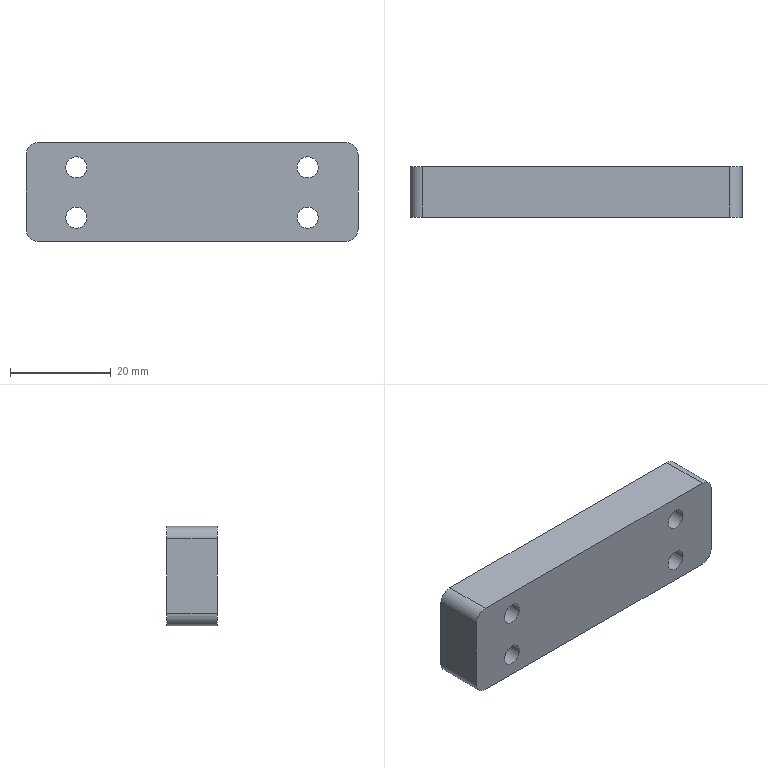Part | SolidWorks | features BaseBody 1 | 1 solid | 18 faces | box 66 x 10 x 19.75 mm | volume 12427 mm3 | cylinder 12 | plane 6 | commonest cylinder face diameters 4.2 x8 5 x4
STEP:
#1=CARTESIAN_POINT('',(-705.131,748.297,332.732));
#2=VERTEX_POINT('',#1);
#3=CARTESIAN_POINT('',(-702.631,748.297,335.232));
#4=VERTEX_POINT('',#3);
#5=CARTESIAN_POINT('',(-705.131,748.297,335.232));
#6=DIRECTION('',(0.,-1.,0.));
#7=DIRECTION('',(0.,0.,-1.));
#8=AXIS2_PLACEMENT_3D('',#5,#6,#7);
#9=CIRCLE('',#8,2.5);
#10=EDGE_CURVE('',#2,#4,#9,.T.);
#11=ORIENTED_EDGE('',*,*,#10,.F.);
#12=CARTESIAN_POINT('',(-766.131,748.297,332.732));
#13=VERTEX_POINT('',#12);
#14=CARTESIAN_POINT('',(-766.131,748.297,332.732));
#15=DIRECTION('',(1.,0.,0.));
#16=VECTOR('',#15,1000.);
#17=LINE('',#14,#16);
#18=EDGE_CURVE('',#13,#2,#17,.T.);
#19=ORIENTED_EDGE('',*,*,#18,.F.);
#20=CARTESIAN_POINT('',(-768.631,748.297,335.232));
#21=VERTEX_POINT('',#20);
#22=CARTESIAN_POINT('',(-766.131,748.297,335.232));
#23=DIRECTION('',(0.,-1.,0.));
#24=DIRECTION('',(-1.,0.,0.));
#25=AXIS2_PLACEMENT_3D('',#22,#23,#24);
#26=CIRCLE('',#25,2.5);
#27=EDGE_CURVE('',#21,#13,#26,.T.);
#28=ORIENTED_EDGE('',*,*,#27,.F.);
#29=CARTESIAN_POINT('',(-768.631,748.297,349.982));
#30=VERTEX_POINT('',#29);
#31=CARTESIAN_POINT('',(-768.631,748.297,349.982));
#32=DIRECTION('',(0.,0.,-1.));
#33=VECTOR('',#32,1000.);
#34=LINE('',#31,#33);
#35=EDGE_CURVE('',#30,#21,#34,.T.);
#36=ORIENTED_EDGE('',*,*,#35,.F.);
#37=CARTESIAN_POINT('',(-766.131,748.297,352.482));
#38=VERTEX_POINT('',#37);
#39=CARTESIAN_POINT('',(-766.131,748.297,349.982));
#40=DIRECTION('',(0.,-1.,0.));
#41=DIRECTION('',(0.,0.,1.));
#42=AXIS2_PLACEMENT_3D('',#39,#40,#41);
#43=CIRCLE('',#42,2.5);
#44=EDGE_CURVE('',#38,#30,#43,.T.);
#45=ORIENTED_EDGE('',*,*,#44,.F.);
#46=CARTESIAN_POINT('',(-705.131,748.297,352.482));
#47=VERTEX_POINT('',#46);
#48=CARTESIAN_POINT('',(-705.131,748.297,352.482));
#49=DIRECTION('',(-1.,0.,0.));
#50=VECTOR('',#49,1000.);
#51=LINE('',#48,#50);
#52=EDGE_CURVE('',#47,#38,#51,.T.);
#53=ORIENTED_EDGE('',*,*,#52,.F.);
#54=CARTESIAN_POINT('',(-702.631,748.297,349.982));
#55=VERTEX_POINT('',#54);
#56=CARTESIAN_POINT('',(-705.131,748.297,349.982));
#57=DIRECTION('',(0.,-1.,0.));
#58=DIRECTION('',(1.,0.,0.));
#59=AXIS2_PLACEMENT_3D('',#56,#57,#58);
#60=CIRCLE('',#59,2.5);
#61=EDGE_CURVE('',#55,#47,#60,.T.);
#62=ORIENTED_EDGE('',*,*,#61,.F.);
#63=CARTESIAN_POINT('',(-702.631,748.297,335.232));
#64=DIRECTION('',(0.,0.,1.));
#65=VECTOR('',#64,1000.);
#66=LINE('',#63,#65);
#67=EDGE_CURVE('',#4,#55,#66,.T.);
#68=ORIENTED_EDGE('',*,*,#67,.F.);
#69=EDGE_LOOP('',(#11,#19,#28,#36,#45,#53,#62,#68));
#70=FACE_OUTER_BOUND('',#69,.T.);
#71=CARTESIAN_POINT('',(-710.531,748.297,347.482));
#72=VERTEX_POINT('',#71);
#73=CARTESIAN_POINT('',(-714.731,748.297,347.482));
#74=VERTEX_POINT('',#73);
#75=CARTESIAN_POINT('',(-712.631,748.297,347.482));
#76=DIRECTION('',(0.,1.,0.));
#77=DIRECTION('',(1.,0.,0.));
#78=AXIS2_PLACEMENT_3D('',#75,#76,#77);
#79=CIRCLE('',#78,2.1);
#80=EDGE_CURVE('',#72,#74,#79,.T.);
#81=ORIENTED_EDGE('',*,*,#80,.F.);
#82=CARTESIAN_POINT('',(-712.631,748.297,347.482));
#83=DIRECTION('',(0.,1.,0.));
#84=DIRECTION('',(-1.,0.,0.));
#85=AXIS2_PLACEMENT_3D('',#82,#83,#84);
#86=CIRCLE('',#85,2.1);
#87=EDGE_CURVE('',#74,#72,#86,.T.);
#88=ORIENTED_EDGE('',*,*,#87,.F.);
#89=EDGE_LOOP('',(#81,#88));
#90=FACE_BOUND('',#89,.T.);
#91=CARTESIAN_POINT('',(-756.531,748.297,347.482));
#92=VERTEX_POINT('',#91);
#93=CARTESIAN_POINT('',(-760.731,748.297,347.482));
#94=VERTEX_POINT('',#93);
#95=CARTESIAN_POINT('',(-758.631,748.297,347.482));
#96=DIRECTION('',(0.,1.,0.));
#97=DIRECTION('',(1.,0.,0.));
#98=AXIS2_PLACEMENT_3D('',#95,#96,#97);
#99=CIRCLE('',#98,2.1);
#100=EDGE_CURVE('',#92,#94,#99,.T.);
#101=ORIENTED_EDGE('',*,*,#100,.F.);
#102=CARTESIAN_POINT('',(-758.631,748.297,347.482));
#103=DIRECTION('',(0.,1.,0.));
#104=DIRECTION('',(-1.,0.,0.));
#105=AXIS2_PLACEMENT_3D('',#102,#103,#104);
#106=CIRCLE('',#105,2.1);
#107=EDGE_CURVE('',#94,#92,#106,.T.);
#108=ORIENTED_EDGE('',*,*,#107,.F.);
#109=EDGE_LOOP('',(#101,#108));
#110=FACE_BOUND('',#109,.T.);
#111=CARTESIAN_POINT('',(-756.531,748.297,337.482));
#112=VERTEX_POINT('',#111);
#113=CARTESIAN_POINT('',(-760.731,748.297,337.482));
#114=VERTEX_POINT('',#113);
#115=CARTESIAN_POINT('',(-758.631,748.297,337.482));
#116=DIRECTION('',(0.,1.,0.));
#117=DIRECTION('',(1.,0.,0.));
#118=AXIS2_PLACEMENT_3D('',#115,#116,#117);
#119=CIRCLE('',#118,2.1);
#120=EDGE_CURVE('',#112,#114,#119,.T.);
#121=ORIENTED_EDGE('',*,*,#120,.F.);
#122=CARTESIAN_POINT('',(-758.631,748.297,337.482));
#123=DIRECTION('',(0.,1.,0.));
#124=DIRECTION('',(-1.,0.,0.));
#125=AXIS2_PLACEMENT_3D('',#122,#123,#124);
#126=CIRCLE('',#125,2.1);
#127=EDGE_CURVE('',#114,#112,#126,.T.);
#128=ORIENTED_EDGE('',*,*,#127,.F.);
#129=EDGE_LOOP('',(#121,#128));
#130=FACE_BOUND('',#129,.T.);
#131=CARTESIAN_POINT('',(-710.531,748.297,337.482));
#132=VERTEX_POINT('',#131);
#133=CARTESIAN_POINT('',(-714.731,748.297,337.482));
#134=VERTEX_POINT('',#133);
#135=CARTESIAN_POINT('',(-712.631,748.297,337.482));
#136=DIRECTION('',(0.,1.,0.));
#137=DIRECTION('',(1.,0.,0.));
#138=AXIS2_PLACEMENT_3D('',#135,#136,#137);
#139=CIRCLE('',#138,2.1);
#140=EDGE_CURVE('',#132,#134,#139,.T.);
#141=ORIENTED_EDGE('',*,*,#140,.F.);
#142=CARTESIAN_POINT('',(-712.631,748.297,337.482));
#143=DIRECTION('',(0.,1.,0.));
#144=DIRECTION('',(-1.,0.,0.));
#145=AXIS2_PLACEMENT_3D('',#142,#143,#144);
#146=CIRCLE('',#145,2.1);
#147=EDGE_CURVE('',#134,#132,#146,.T.);
#148=ORIENTED_EDGE('',*,*,#147,.F.);
#149=EDGE_LOOP('',(#141,#148));
#150=FACE_BOUND('',#149,.T.);
#151=CARTESIAN_POINT('',(-735.631,748.297,352.232));
#152=DIRECTION('',(0.,1.,0.));
#153=DIRECTION('',(-1.,0.,0.));
#154=AXIS2_PLACEMENT_3D('',#151,#152,#153);
#155=PLANE('',#154);
#156=ADVANCED_FACE('',(#70,#90,#110,#130,#150),#155,.T.);
#157=CARTESIAN_POINT('',(-702.631,738.297,335.232));
#158=VERTEX_POINT('',#157);
#159=CARTESIAN_POINT('',(-702.631,738.297,335.232));
#160=DIRECTION('',(0.,1.,0.));
#161=VECTOR('',#160,1000.);
#162=LINE('',#159,#161);
#163=EDGE_CURVE('',#158,#4,#162,.T.);
#164=ORIENTED_EDGE('',*,*,#163,.T.);
#165=ORIENTED_EDGE('',*,*,#67,.T.);
#166=CARTESIAN_POINT('',(-702.631,738.297,349.982));
#167=VERTEX_POINT('',#166);
#168=CARTESIAN_POINT('',(-702.631,748.297,349.982));
#169=DIRECTION('',(0.,-1.,0.));
#170=VECTOR('',#169,1000.);
#171=LINE('',#168,#170);
#172=EDGE_CURVE('',#55,#167,#171,.T.);
#173=ORIENTED_EDGE('',*,*,#172,.T.);
#174=CARTESIAN_POINT('',(-702.631,738.297,349.982));
#175=DIRECTION('',(0.,0.,-1.));
#176=VECTOR('',#175,1000.);
#177=LINE('',#174,#176);
#178=EDGE_CURVE('',#167,#158,#177,.T.);
#179=ORIENTED_EDGE('',*,*,#178,.T.);
#180=EDGE_LOOP('',(#164,#165,#173,#179));
#181=FACE_OUTER_BOUND('',#180,.T.);
#182=CARTESIAN_POINT('',(-702.631,748.297,364.732));
#183=DIRECTION('',(-1.,0.,0.));
#184=DIRECTION('',(0.,-1.,0.));
#185=AXIS2_PLACEMENT_3D('',#182,#183,#184);
#186=PLANE('',#185);
#187=ADVANCED_FACE('',(#181),#186,.F.);
#188=CARTESIAN_POINT('',(-768.631,738.297,349.982));
#189=VERTEX_POINT('',#188);
#190=CARTESIAN_POINT('',(-766.131,738.297,352.482));
#191=VERTEX_POINT('',#190);
#192=CARTESIAN_POINT('',(-766.131,738.297,349.982));
#193=DIRECTION('',(0.,1.,0.));
#194=DIRECTION('',(-1.,0.,0.));
#195=AXIS2_PLACEMENT_3D('',#192,#193,#194);
#196=CIRCLE('',#195,2.5);
#197=EDGE_CURVE('',#189,#191,#196,.T.);
#198=ORIENTED_EDGE('',*,*,#197,.F.);
#199=CARTESIAN_POINT('',(-768.631,738.297,335.232));
#200=VERTEX_POINT('',#199);
#201=CARTESIAN_POINT('',(-768.631,738.297,335.232));
#202=DIRECTION('',(0.,0.,1.));
#203=VECTOR('',#202,1000.);
#204=LINE('',#201,#203);
#205=EDGE_CURVE('',#200,#189,#204,.T.);
#206=ORIENTED_EDGE('',*,*,#205,.F.);
#207=CARTESIAN_POINT('',(-766.131,738.297,332.732));
#208=VERTEX_POINT('',#207);
#209=CARTESIAN_POINT('',(-766.131,738.297,335.232));
#210=DIRECTION('',(0.,1.,0.));
#211=DIRECTION('',(0.,0.,-1.));
#212=AXIS2_PLACEMENT_3D('',#209,#210,#211);
#213=CIRCLE('',#212,2.5);
#214=EDGE_CURVE('',#208,#200,#213,.T.);
#215=ORIENTED_EDGE('',*,*,#214,.F.);
#216=CARTESIAN_POINT('',(-705.131,738.297,332.732));
#217=VERTEX_POINT('',#216);
#218=CARTESIAN_POINT('',(-705.131,738.297,332.732));
#219=DIRECTION('',(-1.,0.,0.));
#220=VECTOR('',#219,1000.);
#221=LINE('',#218,#220);
#222=EDGE_CURVE('',#217,#208,#221,.T.);
#223=ORIENTED_EDGE('',*,*,#222,.F.);
#224=CARTESIAN_POINT('',(-705.131,738.297,335.232));
#225=DIRECTION('',(0.,1.,0.));
#226=DIRECTION('',(1.,0.,0.));
#227=AXIS2_PLACEMENT_3D('',#224,#225,#226);
#228=CIRCLE('',#227,2.5);
#229=EDGE_CURVE('',#158,#217,#228,.T.);
#230=ORIENTED_EDGE('',*,*,#229,.F.);
#231=ORIENTED_EDGE('',*,*,#178,.F.);
#232=CARTESIAN_POINT('',(-705.131,738.297,352.482));
#233=VERTEX_POINT('',#232);
#234=CARTESIAN_POINT('',(-705.131,738.297,349.982));
#235=DIRECTION('',(0.,1.,0.));
#236=DIRECTION('',(0.,0.,1.));
#237=AXIS2_PLACEMENT_3D('',#234,#235,#236);
#238=CIRCLE('',#237,2.5);
#239=EDGE_CURVE('',#233,#167,#238,.T.);
#240=ORIENTED_EDGE('',*,*,#239,.F.);
#241=CARTESIAN_POINT('',(-766.131,738.297,352.482));
#242=DIRECTION('',(1.,0.,0.));
#243=VECTOR('',#242,1000.);
#244=LINE('',#241,#243);
#245=EDGE_CURVE('',#191,#233,#244,.T.);
#246=ORIENTED_EDGE('',*,*,#245,.F.);
#247=EDGE_LOOP('',(#198,#206,#215,#223,#230,#231,#240,#246));
#248=FACE_OUTER_BOUND('',#247,.T.);
#249=CARTESIAN_POINT('',(-714.731,738.297,347.482));
#250=VERTEX_POINT('',#249);
#251=CARTESIAN_POINT('',(-710.531,738.297,347.482));
#252=VERTEX_POINT('',#251);
#253=CARTESIAN_POINT('',(-712.631,738.297,347.482));
#254=DIRECTION('',(0.,-1.,0.));
#255=DIRECTION('',(-1.,0.,0.));
#256=AXIS2_PLACEMENT_3D('',#253,#254,#255);
#257=CIRCLE('',#256,2.1);
#258=EDGE_CURVE('',#250,#252,#257,.T.);
#259=ORIENTED_EDGE('',*,*,#258,.F.);
#260=CARTESIAN_POINT('',(-712.631,738.297,347.482));
#261=DIRECTION('',(0.,-1.,0.));
#262=DIRECTION('',(1.,0.,0.));
#263=AXIS2_PLACEMENT_3D('',#260,#261,#262);
#264=CIRCLE('',#263,2.1);
#265=EDGE_CURVE('',#252,#250,#264,.T.);
#266=ORIENTED_EDGE('',*,*,#265,.F.);
#267=EDGE_LOOP('',(#259,#266));
#268=FACE_BOUND('',#267,.T.);
#269=CARTESIAN_POINT('',(-760.731,738.297,347.482));
#270=VERTEX_POINT('',#269);
#271=CARTESIAN_POINT('',(-756.531,738.297,347.482));
#272=VERTEX_POINT('',#271);
#273=CARTESIAN_POINT('',(-758.631,738.297,347.482));
#274=DIRECTION('',(0.,-1.,0.));
#275=DIRECTION('',(-1.,0.,0.));
#276=AXIS2_PLACEMENT_3D('',#273,#274,#275);
#277=CIRCLE('',#276,2.1);
#278=EDGE_CURVE('',#270,#272,#277,.T.);
#279=ORIENTED_EDGE('',*,*,#278,.F.);
#280=CARTESIAN_POINT('',(-758.631,738.297,347.482));
#281=DIRECTION('',(0.,-1.,0.));
#282=DIRECTION('',(1.,0.,0.));
#283=AXIS2_PLACEMENT_3D('',#280,#281,#282);
#284=CIRCLE('',#283,2.1);
#285=EDGE_CURVE('',#272,#270,#284,.T.);
#286=ORIENTED_EDGE('',*,*,#285,.F.);
#287=EDGE_LOOP('',(#279,#286));
#288=FACE_BOUND('',#287,.T.);
#289=CARTESIAN_POINT('',(-760.731,738.297,337.482));
#290=VERTEX_POINT('',#289);
#291=CARTESIAN_POINT('',(-756.531,738.297,337.482));
#292=VERTEX_POINT('',#291);
#293=CARTESIAN_POINT('',(-758.631,738.297,337.482));
#294=DIRECTION('',(0.,-1.,0.));
#295=DIRECTION('',(-1.,0.,0.));
#296=AXIS2_PLACEMENT_3D('',#293,#294,#295);
#297=CIRCLE('',#296,2.1);
#298=EDGE_CURVE('',#290,#292,#297,.T.);
#299=ORIENTED_EDGE('',*,*,#298,.F.);
#300=CARTESIAN_POINT('',(-758.631,738.297,337.482));
#301=DIRECTION('',(0.,-1.,0.));
#302=DIRECTION('',(1.,0.,0.));
#303=AXIS2_PLACEMENT_3D('',#300,#301,#302);
#304=CIRCLE('',#303,2.1);
#305=EDGE_CURVE('',#292,#290,#304,.T.);
#306=ORIENTED_EDGE('',*,*,#305,.F.);
#307=EDGE_LOOP('',(#299,#306));
#308=FACE_BOUND('',#307,.T.);
#309=CARTESIAN_POINT('',(-714.731,738.297,337.482));
#310=VERTEX_POINT('',#309);
#311=CARTESIAN_POINT('',(-710.531,738.297,337.482));
#312=VERTEX_POINT('',#311);
#313=CARTESIAN_POINT('',(-712.631,738.297,337.482));
#314=DIRECTION('',(0.,-1.,0.));
#315=DIRECTION('',(-1.,0.,0.));
#316=AXIS2_PLACEMENT_3D('',#313,#314,#315);
#317=CIRCLE('',#316,2.1);
#318=EDGE_CURVE('',#310,#312,#317,.T.);
#319=ORIENTED_EDGE('',*,*,#318,.F.);
#320=CARTESIAN_POINT('',(-712.631,738.297,337.482));
#321=DIRECTION('',(0.,-1.,0.));
#322=DIRECTION('',(1.,0.,0.));
#323=AXIS2_PLACEMENT_3D('',#320,#321,#322);
#324=CIRCLE('',#323,2.1);
#325=EDGE_CURVE('',#312,#310,#324,.T.);
#326=ORIENTED_EDGE('',*,*,#325,.F.);
#327=EDGE_LOOP('',(#319,#326));
#328=FACE_BOUND('',#327,.T.);
#329=CARTESIAN_POINT('',(-735.631,738.297,352.232));
#330=DIRECTION('',(0.,1.,0.));
#331=DIRECTION('',(-1.,0.,0.));
#332=AXIS2_PLACEMENT_3D('',#329,#330,#331);
#333=PLANE('',#332);
#334=ADVANCED_FACE('',(#248,#268,#288,#308,#328),#333,.F.);
#335=CARTESIAN_POINT('',(-766.131,748.297,352.482));
#336=DIRECTION('',(0.,-1.,0.));
#337=VECTOR('',#336,1000.);
#338=LINE('',#335,#337);
#339=EDGE_CURVE('',#38,#191,#338,.T.);
#340=ORIENTED_EDGE('',*,*,#339,.T.);
#341=ORIENTED_EDGE('',*,*,#245,.T.);
#342=CARTESIAN_POINT('',(-705.131,738.297,352.482));
#343=DIRECTION('',(0.,1.,0.));
#344=VECTOR('',#343,1000.);
#345=LINE('',#342,#344);
#346=EDGE_CURVE('',#233,#47,#345,.T.);
#347=ORIENTED_EDGE('',*,*,#346,.T.);
#348=ORIENTED_EDGE('',*,*,#52,.T.);
#349=EDGE_LOOP('',(#340,#341,#347,#348));
#350=FACE_OUTER_BOUND('',#349,.T.);
#351=CARTESIAN_POINT('',(-698.167,748.297,352.482));
#352=DIRECTION('',(0.,0.,-1.));
#353=DIRECTION('',(1.,0.,0.));
#354=AXIS2_PLACEMENT_3D('',#351,#352,#353);
#355=PLANE('',#354);
#356=ADVANCED_FACE('',(#350),#355,.F.);
#357=ORIENTED_EDGE('',*,*,#61,.T.);
#358=ORIENTED_EDGE('',*,*,#346,.F.);
#359=ORIENTED_EDGE('',*,*,#239,.T.);
#360=ORIENTED_EDGE('',*,*,#172,.F.);
#361=EDGE_LOOP('',(#357,#358,#359,#360));
#362=FACE_OUTER_BOUND('',#361,.T.);
#363=CARTESIAN_POINT('',(-705.131,761.333,349.982));
#364=DIRECTION('',(0.,-1.,0.));
#365=DIRECTION('',(1.,0.,0.));
#366=AXIS2_PLACEMENT_3D('',#363,#364,#365);
#367=CYLINDRICAL_SURFACE('',#366,2.5);
#368=ADVANCED_FACE('',(#362),#367,.T.);
#369=ORIENTED_EDGE('',*,*,#197,.T.);
#370=ORIENTED_EDGE('',*,*,#339,.F.);
#371=ORIENTED_EDGE('',*,*,#44,.T.);
#372=CARTESIAN_POINT('',(-768.631,738.297,349.982));
#373=DIRECTION('',(0.,1.,0.));
#374=VECTOR('',#373,1000.);
#375=LINE('',#372,#374);
#376=EDGE_CURVE('',#189,#30,#375,.T.);
#377=ORIENTED_EDGE('',*,*,#376,.F.);
#378=EDGE_LOOP('',(#369,#370,#371,#377));
#379=FACE_OUTER_BOUND('',#378,.T.);
#380=CARTESIAN_POINT('',(-766.131,725.261,349.982));
#381=DIRECTION('',(0.,1.,0.));
#382=DIRECTION('',(-1.,0.,0.));
#383=AXIS2_PLACEMENT_3D('',#380,#381,#382);
#384=CYLINDRICAL_SURFACE('',#383,2.5);
#385=ADVANCED_FACE('',(#379),#384,.T.);
#386=CARTESIAN_POINT('',(-768.631,748.297,335.232));
#387=DIRECTION('',(0.,-1.,0.));
#388=VECTOR('',#387,1000.);
#389=LINE('',#386,#388);
#390=EDGE_CURVE('',#21,#200,#389,.T.);
#391=ORIENTED_EDGE('',*,*,#390,.T.);
#392=ORIENTED_EDGE('',*,*,#205,.T.);
#393=ORIENTED_EDGE('',*,*,#376,.T.);
#394=ORIENTED_EDGE('',*,*,#35,.T.);
#395=EDGE_LOOP('',(#391,#392,#393,#394));
#396=FACE_OUTER_BOUND('',#395,.T.);
#397=CARTESIAN_POINT('',(-768.631,748.297,364.732));
#398=DIRECTION('',(1.,0.,0.));
#399=DIRECTION('',(0.,1.,0.));
#400=AXIS2_PLACEMENT_3D('',#397,#398,#399);
#401=PLANE('',#400);
#402=ADVANCED_FACE('',(#396),#401,.F.);
#403=ORIENTED_EDGE('',*,*,#214,.T.);
#404=ORIENTED_EDGE('',*,*,#390,.F.);
#405=ORIENTED_EDGE('',*,*,#27,.T.);
#406=CARTESIAN_POINT('',(-766.131,738.297,332.732));
#407=DIRECTION('',(0.,1.,0.));
#408=VECTOR('',#407,1000.);
#409=LINE('',#406,#408);
#410=EDGE_CURVE('',#208,#13,#409,.T.);
#411=ORIENTED_EDGE('',*,*,#410,.F.);
#412=EDGE_LOOP('',(#403,#404,#405,#411));
#413=FACE_OUTER_BOUND('',#412,.T.);
#414=CARTESIAN_POINT('',(-766.131,725.261,335.232));
#415=DIRECTION('',(0.,1.,0.));
#416=DIRECTION('',(-1.,0.,0.));
#417=AXIS2_PLACEMENT_3D('',#414,#415,#416);
#418=CYLINDRICAL_SURFACE('',#417,2.5);
#419=ADVANCED_FACE('',(#413),#418,.T.);
#420=ORIENTED_EDGE('',*,*,#410,.T.);
#421=ORIENTED_EDGE('',*,*,#18,.T.);
#422=CARTESIAN_POINT('',(-705.131,748.297,332.732));
#423=DIRECTION('',(0.,-1.,0.));
#424=VECTOR('',#423,1000.);
#425=LINE('',#422,#424);
#426=EDGE_CURVE('',#2,#217,#425,.T.);
#427=ORIENTED_EDGE('',*,*,#426,.T.);
#428=ORIENTED_EDGE('',*,*,#222,.T.);
#429=EDGE_LOOP('',(#420,#421,#427,#428));
#430=FACE_OUTER_BOUND('',#429,.T.);
#431=CARTESIAN_POINT('',(-702.631,748.297,332.732));
#432=DIRECTION('',(0.,0.,-1.));
#433=DIRECTION('',(1.,0.,0.));
#434=AXIS2_PLACEMENT_3D('',#431,#432,#433);
#435=PLANE('',#434);
#436=ADVANCED_FACE('',(#430),#435,.T.);
#437=ORIENTED_EDGE('',*,*,#229,.T.);
#438=ORIENTED_EDGE('',*,*,#426,.F.);
#439=ORIENTED_EDGE('',*,*,#10,.T.);
#440=ORIENTED_EDGE('',*,*,#163,.F.);
#441=EDGE_LOOP('',(#437,#438,#439,#440));
#442=FACE_OUTER_BOUND('',#441,.T.);
#443=CARTESIAN_POINT('',(-705.131,725.261,335.232));
#444=DIRECTION('',(0.,1.,0.));
#445=DIRECTION('',(-1.,0.,0.));
#446=AXIS2_PLACEMENT_3D('',#443,#444,#445);
#447=CYLINDRICAL_SURFACE('',#446,2.5);
#448=ADVANCED_FACE('',(#442),#447,.T.);
#449=ORIENTED_EDGE('',*,*,#265,.T.);
#450=CARTESIAN_POINT('',(-714.731,738.297,347.482));
#451=DIRECTION('',(0.,1.,0.));
#452=VECTOR('',#451,1000.);
#453=LINE('',#450,#452);
#454=EDGE_CURVE('',#250,#74,#453,.T.);
#455=ORIENTED_EDGE('',*,*,#454,.T.);
#456=ORIENTED_EDGE('',*,*,#87,.T.);
#457=CARTESIAN_POINT('',(-710.531,748.297,347.482));
#458=DIRECTION('',(0.,-1.,0.));
#459=VECTOR('',#458,1000.);
#460=LINE('',#457,#459);
#461=EDGE_CURVE('',#72,#252,#460,.T.);
#462=ORIENTED_EDGE('',*,*,#461,.T.);
#463=EDGE_LOOP('',(#449,#455,#456,#462));
#464=FACE_OUTER_BOUND('',#463,.T.);
#465=CARTESIAN_POINT('',(-712.631,748.297,347.482));
#466=DIRECTION('',(0.,1.,0.));
#467=DIRECTION('',(-1.,0.,0.));
#468=AXIS2_PLACEMENT_3D('',#465,#466,#467);
#469=CYLINDRICAL_SURFACE('',#468,2.1);
#470=ADVANCED_FACE('',(#464),#469,.F.);
#471=ORIENTED_EDGE('',*,*,#258,.T.);
#472=ORIENTED_EDGE('',*,*,#461,.F.);
#473=ORIENTED_EDGE('',*,*,#80,.T.);
#474=ORIENTED_EDGE('',*,*,#454,.F.);
#475=EDGE_LOOP('',(#471,#472,#473,#474));
#476=FACE_OUTER_BOUND('',#475,.T.);
#477=CARTESIAN_POINT('',(-712.631,748.297,347.482));
#478=DIRECTION('',(0.,1.,0.));
#479=DIRECTION('',(-1.,0.,0.));
#480=AXIS2_PLACEMENT_3D('',#477,#478,#479);
#481=CYLINDRICAL_SURFACE('',#480,2.1);
#482=ADVANCED_FACE('',(#476),#481,.F.);
#483=ORIENTED_EDGE('',*,*,#285,.T.);
#484=CARTESIAN_POINT('',(-760.731,738.297,347.482));
#485=DIRECTION('',(0.,1.,0.));
#486=VECTOR('',#485,1000.);
#487=LINE('',#484,#486);
#488=EDGE_CURVE('',#270,#94,#487,.T.);
#489=ORIENTED_EDGE('',*,*,#488,.T.);
#490=ORIENTED_EDGE('',*,*,#107,.T.);
#491=CARTESIAN_POINT('',(-756.531,748.297,347.482));
#492=DIRECTION('',(0.,-1.,0.));
#493=VECTOR('',#492,1000.);
#494=LINE('',#491,#493);
#495=EDGE_CURVE('',#92,#272,#494,.T.);
#496=ORIENTED_EDGE('',*,*,#495,.T.);
#497=EDGE_LOOP('',(#483,#489,#490,#496));
#498=FACE_OUTER_BOUND('',#497,.T.);
#499=CARTESIAN_POINT('',(-758.631,748.297,347.482));
#500=DIRECTION('',(0.,1.,0.));
#501=DIRECTION('',(-1.,0.,0.));
#502=AXIS2_PLACEMENT_3D('',#499,#500,#501);
#503=CYLINDRICAL_SURFACE('',#502,2.1);
#504=ADVANCED_FACE('',(#498),#503,.F.);
#505=ORIENTED_EDGE('',*,*,#278,.T.);
#506=ORIENTED_EDGE('',*,*,#495,.F.);
#507=ORIENTED_EDGE('',*,*,#100,.T.);
#508=ORIENTED_EDGE('',*,*,#488,.F.);
#509=EDGE_LOOP('',(#505,#506,#507,#508));
#510=FACE_OUTER_BOUND('',#509,.T.);
#511=CARTESIAN_POINT('',(-758.631,748.297,347.482));
#512=DIRECTION('',(0.,1.,0.));
#513=DIRECTION('',(-1.,0.,0.));
#514=AXIS2_PLACEMENT_3D('',#511,#512,#513);
#515=CYLINDRICAL_SURFACE('',#514,2.1);
#516=ADVANCED_FACE('',(#510),#515,.F.);
#517=ORIENTED_EDGE('',*,*,#305,.T.);
#518=CARTESIAN_POINT('',(-760.731,738.297,337.482));
#519=DIRECTION('',(0.,1.,0.));
#520=VECTOR('',#519,1000.);
#521=LINE('',#518,#520);
#522=EDGE_CURVE('',#290,#114,#521,.T.);
#523=ORIENTED_EDGE('',*,*,#522,.T.);
#524=ORIENTED_EDGE('',*,*,#127,.T.);
#525=CARTESIAN_POINT('',(-756.531,748.297,337.482));
#526=DIRECTION('',(0.,-1.,0.));
#527=VECTOR('',#526,1000.);
#528=LINE('',#525,#527);
#529=EDGE_CURVE('',#112,#292,#528,.T.);
#530=ORIENTED_EDGE('',*,*,#529,.T.);
#531=EDGE_LOOP('',(#517,#523,#524,#530));
#532=FACE_OUTER_BOUND('',#531,.T.);
#533=CARTESIAN_POINT('',(-758.631,748.297,337.482));
#534=DIRECTION('',(0.,1.,0.));
#535=DIRECTION('',(-1.,0.,0.));
#536=AXIS2_PLACEMENT_3D('',#533,#534,#535);
#537=CYLINDRICAL_SURFACE('',#536,2.1);
#538=ADVANCED_FACE('',(#532),#537,.F.);
#539=ORIENTED_EDGE('',*,*,#298,.T.);
#540=ORIENTED_EDGE('',*,*,#529,.F.);
#541=ORIENTED_EDGE('',*,*,#120,.T.);
#542=ORIENTED_EDGE('',*,*,#522,.F.);
#543=EDGE_LOOP('',(#539,#540,#541,#542));
#544=FACE_OUTER_BOUND('',#543,.T.);
#545=CARTESIAN_POINT('',(-758.631,748.297,337.482));
#546=DIRECTION('',(0.,1.,0.));
#547=DIRECTION('',(-1.,0.,0.));
#548=AXIS2_PLACEMENT_3D('',#545,#546,#547);
#549=CYLINDRICAL_SURFACE('',#548,2.1);
#550=ADVANCED_FACE('',(#544),#549,.F.);
#551=ORIENTED_EDGE('',*,*,#325,.T.);
#552=CARTESIAN_POINT('',(-714.731,738.297,337.482));
#553=DIRECTION('',(0.,1.,0.));
#554=VECTOR('',#553,1000.);
#555=LINE('',#552,#554);
#556=EDGE_CURVE('',#310,#134,#555,.T.);
#557=ORIENTED_EDGE('',*,*,#556,.T.);
#558=ORIENTED_EDGE('',*,*,#147,.T.);
#559=CARTESIAN_POINT('',(-710.531,748.297,337.482));
#560=DIRECTION('',(0.,-1.,0.));
#561=VECTOR('',#560,1000.);
#562=LINE('',#559,#561);
#563=EDGE_CURVE('',#132,#312,#562,.T.);
#564=ORIENTED_EDGE('',*,*,#563,.T.);
#565=EDGE_LOOP('',(#551,#557,#558,#564));
#566=FACE_OUTER_BOUND('',#565,.T.);
#567=CARTESIAN_POINT('',(-712.631,748.297,337.482));
#568=DIRECTION('',(0.,1.,0.));
#569=DIRECTION('',(-1.,0.,0.));
#570=AXIS2_PLACEMENT_3D('',#567,#568,#569);
#571=CYLINDRICAL_SURFACE('',#570,2.1);
#572=ADVANCED_FACE('',(#566),#571,.F.);
#573=ORIENTED_EDGE('',*,*,#318,.T.);
#574=ORIENTED_EDGE('',*,*,#563,.F.);
#575=ORIENTED_EDGE('',*,*,#140,.T.);
#576=ORIENTED_EDGE('',*,*,#556,.F.);
#577=EDGE_LOOP('',(#573,#574,#575,#576));
#578=FACE_OUTER_BOUND('',#577,.T.);
#579=CARTESIAN_POINT('',(-712.631,748.297,337.482));
#580=DIRECTION('',(0.,1.,0.));
#581=DIRECTION('',(-1.,0.,0.));
#582=AXIS2_PLACEMENT_3D('',#579,#580,#581);
#583=CYLINDRICAL_SURFACE('',#582,2.1);
#584=ADVANCED_FACE('',(#578),#583,.F.);
#585=CLOSED_SHELL('',(#156,#187,#334,#356,#368,#385,#402,#419,#436,#448,#470,#482,#504,#516,#538,#550,#572,#584));
#586=MANIFOLD_SOLID_BREP('',#585);
#587=CARTESIAN_POINT('',(0.,0.,0.));
#588=DIRECTION('',(0.,0.,1.));
#589=DIRECTION('',(1.,0.,0.));
#590=AXIS2_PLACEMENT_3D('',#587,#588,#589);
#591=(LENGTH_UNIT()NAMED_UNIT(*)SI_UNIT(.MILLI.,.METRE.));
#592=UNCERTAINTY_MEASURE_WITH_UNIT(LENGTH_MEASURE(0.00001),#591,'','');
#593=(NAMED_UNIT(*)PLANE_ANGLE_UNIT()SI_UNIT($,.RADIAN.));
#594=(NAMED_UNIT(*)SI_UNIT($,.STERADIAN.)SOLID_ANGLE_UNIT());
#595=(GEOMETRIC_REPRESENTATION_CONTEXT(3)GLOBAL_UNCERTAINTY_ASSIGNED_CONTEXT((#592))GLOBAL_UNIT_ASSIGNED_CONTEXT((#591,#593,#594))REPRESENTATION_CONTEXT('',''));
#596=ADVANCED_BREP_SHAPE_REPRESENTATION('',(#586,#590),#595);